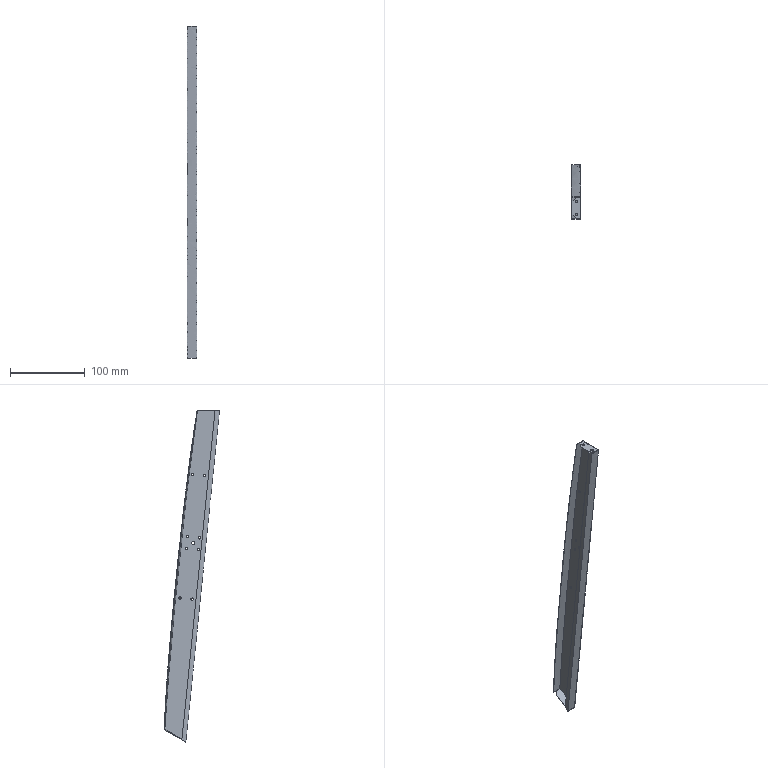Part | SolidWorks | features BaseBody 1 | 1 solid | 43 faces | box 13 x 73.781 x 445.197 mm | volume 15615 mm3 | cylinder 22 | plane 19 | spline 2 | commonest cylinder face diameters 3.2 x20 4.17 x2